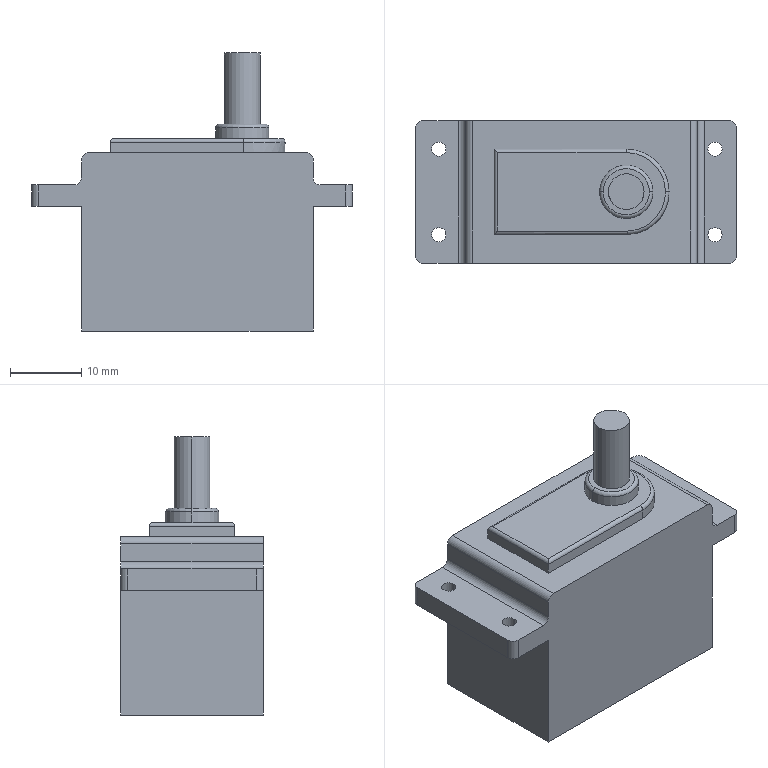Part | SolidWorks | features ICE 6, Fillet 2, Extrusion 1, Scale 1 | 1 solid | 48 faces | box 45 x 20 x 39 mm | volume 17798 mm3 | cylinder 24 | plane 20 | torus 4 | commonest cylinder face diameters 2 x16 1 x3 5 x2 7.5 x2 12 x1
STEP:
#1=CARTESIAN_POINT('',(17.75,6.,17.5));
#2=VERTEX_POINT('',#1);
#3=CARTESIAN_POINT('',(19.75,6.,17.5));
#4=VERTEX_POINT('',#3);
#5=CARTESIAN_POINT('',(18.75,6.,17.5));
#6=DIRECTION('',(0.,0.,1.));
#7=DIRECTION('',(0.,-1.,0.));
#8=AXIS2_PLACEMENT_3D('',#5,#6,#7);
#9=CIRCLE('',#8,1.);
#10=EDGE_CURVE('',#2,#4,#9,.T.);
#11=ORIENTED_EDGE('',*,*,#10,.F.);
#12=CARTESIAN_POINT('',(17.75,6.,20.5));
#13=VERTEX_POINT('',#12);
#14=CARTESIAN_POINT('',(17.75,6.,10.5));
#15=DIRECTION('',(0.,0.,1.));
#16=VECTOR('',#15,1000.);
#17=LINE('',#14,#16);
#18=EDGE_CURVE('',#2,#13,#17,.T.);
#19=ORIENTED_EDGE('',*,*,#18,.T.);
#20=CARTESIAN_POINT('',(19.75,6.,20.5));
#21=VERTEX_POINT('',#20);
#22=CARTESIAN_POINT('',(18.75,6.,20.5));
#23=DIRECTION('',(0.,0.,1.));
#24=DIRECTION('',(1.,0.,0.));
#25=AXIS2_PLACEMENT_3D('',#22,#23,#24);
#26=CIRCLE('',#25,1.);
#27=EDGE_CURVE('',#13,#21,#26,.T.);
#28=ORIENTED_EDGE('',*,*,#27,.T.);
#29=CARTESIAN_POINT('',(19.75,6.,10.5));
#30=DIRECTION('',(0.,0.,1.));
#31=VECTOR('',#30,1000.);
#32=LINE('',#29,#31);
#33=EDGE_CURVE('',#4,#21,#32,.T.);
#34=ORIENTED_EDGE('',*,*,#33,.F.);
#35=EDGE_LOOP('',(#11,#19,#28,#34));
#36=FACE_OUTER_BOUND('',#35,.T.);
#37=CARTESIAN_POINT('',(18.75,6.,10.5));
#38=DIRECTION('',(0.,0.,1.));
#39=DIRECTION('',(1.,0.,0.));
#40=AXIS2_PLACEMENT_3D('',#37,#38,#39);
#41=CYLINDRICAL_SURFACE('',#40,1.);
#42=ADVANCED_FACE('',(#36),#41,.F.);
#43=CARTESIAN_POINT('',(17.75,-6.,17.5));
#44=VERTEX_POINT('',#43);
#45=CARTESIAN_POINT('',(19.75,-6.,17.5));
#46=VERTEX_POINT('',#45);
#47=CARTESIAN_POINT('',(18.75,-6.,17.5));
#48=DIRECTION('',(0.,0.,1.));
#49=DIRECTION('',(0.,-1.,0.));
#50=AXIS2_PLACEMENT_3D('',#47,#48,#49);
#51=CIRCLE('',#50,1.);
#52=EDGE_CURVE('',#44,#46,#51,.T.);
#53=ORIENTED_EDGE('',*,*,#52,.F.);
#54=CARTESIAN_POINT('',(17.75,-6.,20.5));
#55=VERTEX_POINT('',#54);
#56=CARTESIAN_POINT('',(17.75,-6.,10.5));
#57=DIRECTION('',(0.,0.,1.));
#58=VECTOR('',#57,1000.);
#59=LINE('',#56,#58);
#60=EDGE_CURVE('',#44,#55,#59,.T.);
#61=ORIENTED_EDGE('',*,*,#60,.T.);
#62=CARTESIAN_POINT('',(19.75,-6.,20.5));
#63=VERTEX_POINT('',#62);
#64=CARTESIAN_POINT('',(18.75,-6.,20.5));
#65=DIRECTION('',(0.,0.,1.));
#66=DIRECTION('',(1.,0.,0.));
#67=AXIS2_PLACEMENT_3D('',#64,#65,#66);
#68=CIRCLE('',#67,1.);
#69=EDGE_CURVE('',#55,#63,#68,.T.);
#70=ORIENTED_EDGE('',*,*,#69,.T.);
#71=CARTESIAN_POINT('',(19.75,-6.,10.5));
#72=DIRECTION('',(0.,0.,1.));
#73=VECTOR('',#72,1000.);
#74=LINE('',#71,#73);
#75=EDGE_CURVE('',#46,#63,#74,.T.);
#76=ORIENTED_EDGE('',*,*,#75,.F.);
#77=EDGE_LOOP('',(#53,#61,#70,#76));
#78=FACE_OUTER_BOUND('',#77,.T.);
#79=CARTESIAN_POINT('',(18.75,-6.,10.5));
#80=DIRECTION('',(0.,0.,1.));
#81=DIRECTION('',(1.,0.,0.));
#82=AXIS2_PLACEMENT_3D('',#79,#80,#81);
#83=CYLINDRICAL_SURFACE('',#82,1.);
#84=ADVANCED_FACE('',(#78),#83,.F.);
#85=CARTESIAN_POINT('',(-20.99,-6.,17.5));
#86=VERTEX_POINT('',#85);
#87=CARTESIAN_POINT('',(-18.99,-6.,17.5));
#88=VERTEX_POINT('',#87);
#89=CARTESIAN_POINT('',(-19.99,-6.,17.5));
#90=DIRECTION('',(0.,0.,1.));
#91=DIRECTION('',(0.,-1.,0.));
#92=AXIS2_PLACEMENT_3D('',#89,#90,#91);
#93=CIRCLE('',#92,1.);
#94=EDGE_CURVE('',#86,#88,#93,.T.);
#95=ORIENTED_EDGE('',*,*,#94,.F.);
#96=CARTESIAN_POINT('',(-20.99,-6.,20.5));
#97=VERTEX_POINT('',#96);
#98=CARTESIAN_POINT('',(-20.99,-6.,10.5));
#99=DIRECTION('',(0.,0.,1.));
#100=VECTOR('',#99,1000.);
#101=LINE('',#98,#100);
#102=EDGE_CURVE('',#86,#97,#101,.T.);
#103=ORIENTED_EDGE('',*,*,#102,.T.);
#104=CARTESIAN_POINT('',(-18.99,-6.,20.5));
#105=VERTEX_POINT('',#104);
#106=CARTESIAN_POINT('',(-19.99,-6.,20.5));
#107=DIRECTION('',(0.,0.,1.));
#108=DIRECTION('',(1.,0.,0.));
#109=AXIS2_PLACEMENT_3D('',#106,#107,#108);
#110=CIRCLE('',#109,1.);
#111=EDGE_CURVE('',#97,#105,#110,.T.);
#112=ORIENTED_EDGE('',*,*,#111,.T.);
#113=CARTESIAN_POINT('',(-18.99,-6.,10.5));
#114=DIRECTION('',(0.,0.,1.));
#115=VECTOR('',#114,1000.);
#116=LINE('',#113,#115);
#117=EDGE_CURVE('',#88,#105,#116,.T.);
#118=ORIENTED_EDGE('',*,*,#117,.F.);
#119=EDGE_LOOP('',(#95,#103,#112,#118));
#120=FACE_OUTER_BOUND('',#119,.T.);
#121=CARTESIAN_POINT('',(-19.99,-6.,10.5));
#122=DIRECTION('',(0.,0.,1.));
#123=DIRECTION('',(1.,0.,0.));
#124=AXIS2_PLACEMENT_3D('',#121,#122,#123);
#125=CYLINDRICAL_SURFACE('',#124,1.);
#126=ADVANCED_FACE('',(#120),#125,.F.);
#127=CARTESIAN_POINT('',(-20.99,6.,17.5));
#128=VERTEX_POINT('',#127);
#129=CARTESIAN_POINT('',(-18.99,6.,17.5));
#130=VERTEX_POINT('',#129);
#131=CARTESIAN_POINT('',(-19.99,6.,17.5));
#132=DIRECTION('',(0.,0.,1.));
#133=DIRECTION('',(0.,-1.,0.));
#134=AXIS2_PLACEMENT_3D('',#131,#132,#133);
#135=CIRCLE('',#134,1.);
#136=EDGE_CURVE('',#128,#130,#135,.T.);
#137=ORIENTED_EDGE('',*,*,#136,.F.);
#138=CARTESIAN_POINT('',(-20.99,6.,20.5));
#139=VERTEX_POINT('',#138);
#140=CARTESIAN_POINT('',(-20.99,6.,10.5));
#141=DIRECTION('',(0.,0.,1.));
#142=VECTOR('',#141,1000.);
#143=LINE('',#140,#142);
#144=EDGE_CURVE('',#128,#139,#143,.T.);
#145=ORIENTED_EDGE('',*,*,#144,.T.);
#146=CARTESIAN_POINT('',(-18.99,6.,20.5));
#147=VERTEX_POINT('',#146);
#148=CARTESIAN_POINT('',(-19.99,6.,20.5));
#149=DIRECTION('',(0.,0.,1.));
#150=DIRECTION('',(1.,0.,0.));
#151=AXIS2_PLACEMENT_3D('',#148,#149,#150);
#152=CIRCLE('',#151,1.);
#153=EDGE_CURVE('',#139,#147,#152,.T.);
#154=ORIENTED_EDGE('',*,*,#153,.T.);
#155=CARTESIAN_POINT('',(-18.99,6.,10.5));
#156=DIRECTION('',(0.,0.,1.));
#157=VECTOR('',#156,1000.);
#158=LINE('',#155,#157);
#159=EDGE_CURVE('',#130,#147,#158,.T.);
#160=ORIENTED_EDGE('',*,*,#159,.F.);
#161=EDGE_LOOP('',(#137,#145,#154,#160));
#162=FACE_OUTER_BOUND('',#161,.T.);
#163=CARTESIAN_POINT('',(-19.99,6.,10.5));
#164=DIRECTION('',(0.,0.,1.));
#165=DIRECTION('',(1.,0.,0.));
#166=AXIS2_PLACEMENT_3D('',#163,#164,#165);
#167=CYLINDRICAL_SURFACE('',#166,1.);
#168=ADVANCED_FACE('',(#162),#167,.F.);
#169=CARTESIAN_POINT('',(2.551,0.,28.5));
#170=VERTEX_POINT('',#169);
#171=CARTESIAN_POINT('',(10.051,0.,28.5));
#172=VERTEX_POINT('',#171);
#173=CARTESIAN_POINT('',(6.301,0.,28.5));
#174=DIRECTION('',(0.,0.,-1.));
#175=DIRECTION('',(1.,0.,0.));
#176=AXIS2_PLACEMENT_3D('',#173,#174,#175);
#177=CIRCLE('',#176,3.75);
#178=EDGE_CURVE('',#170,#172,#177,.T.);
#179=ORIENTED_EDGE('',*,*,#178,.F.);
#180=CARTESIAN_POINT('',(3.051,0.,29.));
#181=VERTEX_POINT('',#180);
#182=CARTESIAN_POINT('',(3.051,0.,28.5));
#183=DIRECTION('',(0.,1.,0.));
#184=DIRECTION('',(-1.,0.,0.));
#185=AXIS2_PLACEMENT_3D('',#182,#183,#184);
#186=CIRCLE('',#185,0.5);
#187=EDGE_CURVE('',#170,#181,#186,.T.);
#188=ORIENTED_EDGE('',*,*,#187,.T.);
#189=CARTESIAN_POINT('',(9.551,0.,29.));
#190=VERTEX_POINT('',#189);
#191=CARTESIAN_POINT('',(6.301,0.,29.));
#192=DIRECTION('',(0.,0.,1.));
#193=DIRECTION('',(1.,0.,0.));
#194=AXIS2_PLACEMENT_3D('',#191,#192,#193);
#195=CIRCLE('',#194,3.25);
#196=EDGE_CURVE('',#190,#181,#195,.T.);
#197=ORIENTED_EDGE('',*,*,#196,.F.);
#198=CARTESIAN_POINT('',(9.551,0.,28.5));
#199=DIRECTION('',(0.,-1.,0.));
#200=DIRECTION('',(0.,0.,-1.));
#201=AXIS2_PLACEMENT_3D('',#198,#199,#200);
#202=CIRCLE('',#201,0.5);
#203=EDGE_CURVE('',#172,#190,#202,.T.);
#204=ORIENTED_EDGE('',*,*,#203,.F.);
#205=EDGE_LOOP('',(#179,#188,#197,#204));
#206=FACE_OUTER_BOUND('',#205,.T.);
#207=CARTESIAN_POINT('',(6.301,0.,28.5));
#208=DIRECTION('',(0.,0.,1.));
#209=DIRECTION('',(1.,0.,0.));
#210=AXIS2_PLACEMENT_3D('',#207,#208,#209);
#211=TOROIDAL_SURFACE('',#210,3.25,0.5);
#212=ADVANCED_FACE('',(#206),#211,.T.);
#213=CARTESIAN_POINT('',(12.301,0.,26.5));
#214=VERTEX_POINT('',#213);
#215=CARTESIAN_POINT('',(6.498,-5.997,26.5));
#216=VERTEX_POINT('',#215);
#217=CARTESIAN_POINT('',(6.301,0.,26.5));
#218=DIRECTION('',(0.,0.,-1.));
#219=DIRECTION('',(1.,0.,0.));
#220=AXIS2_PLACEMENT_3D('',#217,#218,#219);
#221=CIRCLE('',#220,6.);
#222=EDGE_CURVE('',#214,#216,#221,.T.);
#223=ORIENTED_EDGE('',*,*,#222,.F.);
#224=CARTESIAN_POINT('',(11.801,0.,27.));
#225=VERTEX_POINT('',#224);
#226=CARTESIAN_POINT('',(11.801,0.,26.5));
#227=DIRECTION('',(0.,-1.,0.));
#228=DIRECTION('',(0.,0.,-1.));
#229=AXIS2_PLACEMENT_3D('',#226,#227,#228);
#230=CIRCLE('',#229,0.5);
#231=EDGE_CURVE('',#214,#225,#230,.T.);
#232=ORIENTED_EDGE('',*,*,#231,.T.);
#233=CARTESIAN_POINT('',(6.489,-5.497,27.));
#234=VERTEX_POINT('',#233);
#235=CARTESIAN_POINT('',(6.301,0.,27.));
#236=DIRECTION('',(0.,0.,1.));
#237=DIRECTION('',(1.,0.,0.));
#238=AXIS2_PLACEMENT_3D('',#235,#236,#237);
#239=CIRCLE('',#238,5.5);
#240=EDGE_CURVE('',#234,#225,#239,.T.);
#241=ORIENTED_EDGE('',*,*,#240,.F.);
#242=CARTESIAN_POINT('',(6.489,-5.497,27.));
#243=CARTESIAN_POINT('',(6.492,-5.628,27.));
#244=CARTESIAN_POINT('',(6.494,-5.758,26.946));
#245=CARTESIAN_POINT('',(6.497,-5.943,26.761));
#246=CARTESIAN_POINT('',(6.498,-5.997,26.632));
#247=CARTESIAN_POINT('',(6.498,-5.997,26.5));
#248=B_SPLINE_CURVE_WITH_KNOTS('',3,(#242,#243,#244,#245,#246,#247),.UNSPECIFIED.,.F.,.F.,(4,2,4),(-0.00001713,0.0003773,0.0007717),.UNSPECIFIED.);
#249=EDGE_CURVE('',#234,#216,#248,.T.);
#250=ORIENTED_EDGE('',*,*,#249,.T.);
#251=EDGE_LOOP('',(#223,#232,#241,#250));
#252=FACE_OUTER_BOUND('',#251,.T.);
#253=CARTESIAN_POINT('',(6.301,0.,26.5));
#254=DIRECTION('',(0.,0.,1.));
#255=DIRECTION('',(1.,0.,0.));
#256=AXIS2_PLACEMENT_3D('',#253,#254,#255);
#257=TOROIDAL_SURFACE('',#256,5.5,0.5);
#258=ADVANCED_FACE('',(#252),#257,.T.);
#259=CARTESIAN_POINT('',(8.801,0.,39.));
#260=VERTEX_POINT('',#259);
#261=CARTESIAN_POINT('',(3.801,0.,39.));
#262=VERTEX_POINT('',#261);
#263=CARTESIAN_POINT('',(6.301,0.,39.));
#264=DIRECTION('',(0.,0.,1.));
#265=DIRECTION('',(1.,0.,0.));
#266=AXIS2_PLACEMENT_3D('',#263,#264,#265);
#267=CIRCLE('',#266,2.5);
#268=EDGE_CURVE('',#260,#262,#267,.T.);
#269=ORIENTED_EDGE('',*,*,#268,.F.);
#270=CARTESIAN_POINT('',(8.801,0.,29.));
#271=VERTEX_POINT('',#270);
#272=CARTESIAN_POINT('',(8.801,0.,39.));
#273=DIRECTION('',(0.,0.,-1.));
#274=VECTOR('',#273,1000.);
#275=LINE('',#272,#274);
#276=EDGE_CURVE('',#260,#271,#275,.T.);
#277=ORIENTED_EDGE('',*,*,#276,.T.);
#278=CARTESIAN_POINT('',(3.801,0.,29.));
#279=VERTEX_POINT('',#278);
#280=CARTESIAN_POINT('',(6.301,0.,29.));
#281=DIRECTION('',(0.,0.,1.));
#282=DIRECTION('',(1.,0.,0.));
#283=AXIS2_PLACEMENT_3D('',#280,#281,#282);
#284=CIRCLE('',#283,2.5);
#285=EDGE_CURVE('',#271,#279,#284,.T.);
#286=ORIENTED_EDGE('',*,*,#285,.T.);
#287=CARTESIAN_POINT('',(3.801,0.,39.));
#288=DIRECTION('',(0.,0.,-1.));
#289=VECTOR('',#288,1000.);
#290=LINE('',#287,#289);
#291=EDGE_CURVE('',#262,#279,#290,.T.);
#292=ORIENTED_EDGE('',*,*,#291,.F.);
#293=EDGE_LOOP('',(#269,#277,#286,#292));
#294=FACE_OUTER_BOUND('',#293,.T.);
#295=CARTESIAN_POINT('',(6.301,0.,39.));
#296=DIRECTION('',(0.,0.,-1.));
#297=DIRECTION('',(-1.,0.,0.));
#298=AXIS2_PLACEMENT_3D('',#295,#296,#297);
#299=CYLINDRICAL_SURFACE('',#298,2.5);
#300=ADVANCED_FACE('',(#294),#299,.T.);
#301=ORIENTED_EDGE('',*,*,#178,.T.);
#302=CARTESIAN_POINT('',(10.051,0.,27.));
#303=VERTEX_POINT('',#302);
#304=CARTESIAN_POINT('',(10.051,0.,29.));
#305=DIRECTION('',(0.,0.,-1.));
#306=VECTOR('',#305,1000.);
#307=LINE('',#304,#306);
#308=EDGE_CURVE('',#172,#303,#307,.T.);
#309=ORIENTED_EDGE('',*,*,#308,.T.);
#310=CARTESIAN_POINT('',(2.551,0.,27.));
#311=VERTEX_POINT('',#310);
#312=CARTESIAN_POINT('',(6.301,0.,27.));
#313=DIRECTION('',(0.,0.,1.));
#314=DIRECTION('',(1.,0.,0.));
#315=AXIS2_PLACEMENT_3D('',#312,#313,#314);
#316=CIRCLE('',#315,3.75);
#317=EDGE_CURVE('',#303,#311,#316,.T.);
#318=ORIENTED_EDGE('',*,*,#317,.T.);
#319=CARTESIAN_POINT('',(2.551,0.,29.));
#320=DIRECTION('',(0.,0.,-1.));
#321=VECTOR('',#320,1000.);
#322=LINE('',#319,#321);
#323=EDGE_CURVE('',#170,#311,#322,.T.);
#324=ORIENTED_EDGE('',*,*,#323,.F.);
#325=EDGE_LOOP('',(#301,#309,#318,#324));
#326=FACE_OUTER_BOUND('',#325,.T.);
#327=CARTESIAN_POINT('',(6.301,0.,29.));
#328=DIRECTION('',(0.,0.,-1.));
#329=DIRECTION('',(-1.,0.,0.));
#330=AXIS2_PLACEMENT_3D('',#327,#328,#329);
#331=CYLINDRICAL_SURFACE('',#330,3.75);
#332=ADVANCED_FACE('',(#326),#331,.T.);
#333=CARTESIAN_POINT('',(-16.25,10.,24.));
#334=VERTEX_POINT('',#333);
#335=CARTESIAN_POINT('',(-16.25,10.,21.5));
#336=VERTEX_POINT('',#335);
#337=CARTESIAN_POINT('',(-16.25,10.,25.));
#338=DIRECTION('',(0.,0.,-1.));
#339=VECTOR('',#338,1000.);
#340=LINE('',#337,#339);
#341=EDGE_CURVE('',#334,#336,#340,.T.);
#342=ORIENTED_EDGE('',*,*,#341,.T.);
#343=CARTESIAN_POINT('',(-16.25,-10.,21.5));
#344=VERTEX_POINT('',#343);
#345=CARTESIAN_POINT('',(-16.25,-10.,21.5));
#346=DIRECTION('',(0.,-1.,0.));
#347=VECTOR('',#346,1000.);
#348=LINE('',#345,#347);
#349=EDGE_CURVE('',#336,#344,#348,.T.);
#350=ORIENTED_EDGE('',*,*,#349,.T.);
#351=CARTESIAN_POINT('',(-16.25,-10.,24.));
#352=VERTEX_POINT('',#351);
#353=CARTESIAN_POINT('',(-16.25,-10.,25.));
#354=DIRECTION('',(0.,0.,-1.));
#355=VECTOR('',#354,1000.);
#356=LINE('',#353,#355);
#357=EDGE_CURVE('',#352,#344,#356,.T.);
#358=ORIENTED_EDGE('',*,*,#357,.F.);
#359=CARTESIAN_POINT('',(-16.25,10.,24.));
#360=DIRECTION('',(0.,1.,0.));
#361=VECTOR('',#360,1000.);
#362=LINE('',#359,#361);
#363=EDGE_CURVE('',#352,#334,#362,.T.);
#364=ORIENTED_EDGE('',*,*,#363,.T.);
#365=EDGE_LOOP('',(#342,#350,#358,#364));
#366=FACE_OUTER_BOUND('',#365,.T.);
#367=CARTESIAN_POINT('',(-16.25,-10.,25.));
#368=DIRECTION('',(1.,0.,0.));
#369=DIRECTION('',(0.,0.,-1.));
#370=AXIS2_PLACEMENT_3D('',#367,#368,#369);
#371=PLANE('',#370);
#372=ADVANCED_FACE('',(#366),#371,.F.);
#373=CARTESIAN_POINT('',(-16.25,10.,17.5));
#374=VERTEX_POINT('',#373);
#375=CARTESIAN_POINT('',(-16.25,-10.,17.5));
#376=VERTEX_POINT('',#375);
#377=CARTESIAN_POINT('',(-16.25,10.,17.5));
#378=DIRECTION('',(0.,-1.,0.));
#379=VECTOR('',#378,1000.);
#380=LINE('',#377,#379);
#381=EDGE_CURVE('',#374,#376,#380,.T.);
#382=ORIENTED_EDGE('',*,*,#381,.F.);
#383=CARTESIAN_POINT('',(-16.25,10.,0.));
#384=VERTEX_POINT('',#383);
#385=CARTESIAN_POINT('',(-16.25,10.,25.));
#386=DIRECTION('',(0.,0.,-1.));
#387=VECTOR('',#386,1000.);
#388=LINE('',#385,#387);
#389=EDGE_CURVE('',#374,#384,#388,.T.);
#390=ORIENTED_EDGE('',*,*,#389,.T.);
#391=CARTESIAN_POINT('',(-16.25,-10.,0.));
#392=VERTEX_POINT('',#391);
#393=CARTESIAN_POINT('',(-16.25,-10.,0.));
#394=DIRECTION('',(0.,-1.,0.));
#395=VECTOR('',#394,1000.);
#396=LINE('',#393,#395);
#397=EDGE_CURVE('',#384,#392,#396,.T.);
#398=ORIENTED_EDGE('',*,*,#397,.T.);
#399=CARTESIAN_POINT('',(-16.25,-10.,25.));
#400=DIRECTION('',(0.,0.,-1.));
#401=VECTOR('',#400,1000.);
#402=LINE('',#399,#401);
#403=EDGE_CURVE('',#376,#392,#402,.T.);
#404=ORIENTED_EDGE('',*,*,#403,.F.);
#405=EDGE_LOOP('',(#382,#390,#398,#404));
#406=FACE_OUTER_BOUND('',#405,.T.);
#407=CARTESIAN_POINT('',(-16.25,-10.,25.));
#408=DIRECTION('',(1.,0.,0.));
#409=DIRECTION('',(0.,0.,-1.));
#410=AXIS2_PLACEMENT_3D('',#407,#408,#409);
#411=PLANE('',#410);
#412=ADVANCED_FACE('',(#406),#411,.F.);
#413=CARTESIAN_POINT('',(16.25,-10.,24.));
#414=VERTEX_POINT('',#413);
#415=CARTESIAN_POINT('',(16.25,-10.,21.5));
#416=VERTEX_POINT('',#415);
#417=CARTESIAN_POINT('',(16.25,-10.,25.));
#418=DIRECTION('',(0.,0.,-1.));
#419=VECTOR('',#418,1000.);
#420=LINE('',#417,#419);
#421=EDGE_CURVE('',#414,#416,#420,.T.);
#422=ORIENTED_EDGE('',*,*,#421,.T.);
#423=CARTESIAN_POINT('',(16.25,10.,21.5));
#424=VERTEX_POINT('',#423);
#425=CARTESIAN_POINT('',(16.25,10.,21.5));
#426=DIRECTION('',(0.,1.,0.));
#427=VECTOR('',#426,1000.);
#428=LINE('',#425,#427);
#429=EDGE_CURVE('',#416,#424,#428,.T.);
#430=ORIENTED_EDGE('',*,*,#429,.T.);
#431=CARTESIAN_POINT('',(16.25,10.,24.));
#432=VERTEX_POINT('',#431);
#433=CARTESIAN_POINT('',(16.25,10.,25.));
#434=DIRECTION('',(0.,0.,-1.));
#435=VECTOR('',#434,1000.);
#436=LINE('',#433,#435);
#437=EDGE_CURVE('',#432,#424,#436,.T.);
#438=ORIENTED_EDGE('',*,*,#437,.F.);
#439=CARTESIAN_POINT('',(16.25,-10.,24.));
#440=DIRECTION('',(0.,-1.,0.));
#441=VECTOR('',#440,1000.);
#442=LINE('',#439,#441);
#443=EDGE_CURVE('',#432,#414,#442,.T.);
#444=ORIENTED_EDGE('',*,*,#443,.T.);
#445=EDGE_LOOP('',(#422,#430,#438,#444));
#446=FACE_OUTER_BOUND('',#445,.T.);
#447=CARTESIAN_POINT('',(16.25,-10.,25.));
#448=DIRECTION('',(-1.,0.,0.));
#449=DIRECTION('',(0.,0.,1.));
#450=AXIS2_PLACEMENT_3D('',#447,#448,#449);
#451=PLANE('',#450);
#452=ADVANCED_FACE('',(#446),#451,.F.);
#453=CARTESIAN_POINT('',(16.25,-10.,17.5));
#454=VERTEX_POINT('',#453);
#455=CARTESIAN_POINT('',(16.25,10.,17.5));
#456=VERTEX_POINT('',#455);
#457=CARTESIAN_POINT('',(16.25,10.,17.5));
#458=DIRECTION('',(0.,1.,0.));
#459=VECTOR('',#458,1000.);
#460=LINE('',#457,#459);
#461=EDGE_CURVE('',#454,#456,#460,.T.);
#462=ORIENTED_EDGE('',*,*,#461,.F.);
#463=CARTESIAN_POINT('',(16.25,-10.,0.));
#464=VERTEX_POINT('',#463);
#465=CARTESIAN_POINT('',(16.25,-10.,25.));
#466=DIRECTION('',(0.,0.,-1.));
#467=VECTOR('',#466,1000.);
#468=LINE('',#465,#467);
#469=EDGE_CURVE('',#454,#464,#468,.T.);
#470=ORIENTED_EDGE('',*,*,#469,.T.);
#471=CARTESIAN_POINT('',(16.25,10.,0.));
#472=VERTEX_POINT('',#471);
#473=CARTESIAN_POINT('',(16.25,-10.,0.));
#474=DIRECTION('',(0.,1.,0.));
#475=VECTOR('',#474,1000.);
#476=LINE('',#473,#475);
#477=EDGE_CURVE('',#464,#472,#476,.T.);
#478=ORIENTED_EDGE('',*,*,#477,.T.);
#479=CARTESIAN_POINT('',(16.25,10.,25.));
#480=DIRECTION('',(0.,0.,-1.));
#481=VECTOR('',#480,1000.);
#482=LINE('',#479,#481);
#483=EDGE_CURVE('',#456,#472,#482,.T.);
#484=ORIENTED_EDGE('',*,*,#483,.F.);
#485=EDGE_LOOP('',(#462,#470,#478,#484));
#486=FACE_OUTER_BOUND('',#485,.T.);
#487=CARTESIAN_POINT('',(16.25,-10.,25.));
#488=DIRECTION('',(-1.,0.,0.));
#489=DIRECTION('',(0.,0.,1.));
#490=AXIS2_PLACEMENT_3D('',#487,#488,#489);
#491=PLANE('',#490);
#492=ADVANCED_FACE('',(#486),#491,.F.);
#493=ORIENTED_EDGE('',*,*,#421,.F.);
#494=CARTESIAN_POINT('',(15.25,-10.,25.));
#495=VERTEX_POINT('',#494);
#496=CARTESIAN_POINT('',(15.25,-10.,24.));
#497=DIRECTION('',(0.,-1.,0.));
#498=DIRECTION('',(-1.,0.,0.));
#499=AXIS2_PLACEMENT_3D('',#496,#497,#498);
#500=CIRCLE('',#499,1.);
#501=EDGE_CURVE('',#414,#495,#500,.T.);
#502=ORIENTED_EDGE('',*,*,#501,.T.);
#503=CARTESIAN_POINT('',(-15.25,-10.,25.));
#504=VERTEX_POINT('',#503);
#505=CARTESIAN_POINT('',(16.25,-10.,25.));
#506=DIRECTION('',(1.,0.,0.));
#507=VECTOR('',#506,1000.);
#508=LINE('',#505,#507);
#509=EDGE_CURVE('',#504,#495,#508,.T.);
#510=ORIENTED_EDGE('',*,*,#509,.F.);
#511=CARTESIAN_POINT('',(-15.25,-10.,24.));
#512=DIRECTION('',(0.,-1.,0.));
#513=DIRECTION('',(-1.,0.,0.));
#514=AXIS2_PLACEMENT_3D('',#511,#512,#513);
#515=CIRCLE('',#514,1.);
#516=EDGE_CURVE('',#504,#352,#515,.T.);
#517=ORIENTED_EDGE('',*,*,#516,.T.);
#518=ORIENTED_EDGE('',*,*,#357,.T.);
#519=CARTESIAN_POINT('',(-17.25,-10.,20.5));
#520=VERTEX_POINT('',#519);
#521=CARTESIAN_POINT('',(-17.25,-10.,21.5));
#522=DIRECTION('',(0.,1.,0.));
#523=DIRECTION('',(-1.,0.,0.));
#524=AXIS2_PLACEMENT_3D('',#521,#522,#523);
#525=CIRCLE('',#524,1.);
#526=EDGE_CURVE('',#344,#520,#525,.T.);
#527=ORIENTED_EDGE('',*,*,#526,.T.);
#528=CARTESIAN_POINT('',(-22.25,-10.,20.5));
#529=VERTEX_POINT('',#528);
#530=CARTESIAN_POINT('',(-26.25,-10.,20.5));
#531=DIRECTION('',(1.,0.,0.));
#532=VECTOR('',#531,1000.);
#533=LINE('',#530,#532);
#534=EDGE_CURVE('',#529,#520,#533,.T.);
#535=ORIENTED_EDGE('',*,*,#534,.F.);
#536=CARTESIAN_POINT('',(-22.25,-10.,17.5));
#537=VERTEX_POINT('',#536);
#538=CARTESIAN_POINT('',(-22.25,-10.,25.));
#539=DIRECTION('',(0.,0.,-1.));
#540=VECTOR('',#539,1000.);
#541=LINE('',#538,#540);
#542=EDGE_CURVE('',#529,#537,#541,.T.);
#543=ORIENTED_EDGE('',*,*,#542,.T.);
#544=CARTESIAN_POINT('',(-26.25,-10.,17.5));
#545=DIRECTION('',(1.,0.,0.));
#546=VECTOR('',#545,1000.);
#547=LINE('',#544,#546);
#548=EDGE_CURVE('',#537,#376,#547,.T.);
#549=ORIENTED_EDGE('',*,*,#548,.T.);
#550=ORIENTED_EDGE('',*,*,#403,.T.);
#551=CARTESIAN_POINT('',(16.25,-10.,0.));
#552=DIRECTION('',(1.,0.,0.));
#553=VECTOR('',#552,1000.);
#554=LINE('',#551,#553);
#555=EDGE_CURVE('',#392,#464,#554,.T.);
#556=ORIENTED_EDGE('',*,*,#555,.T.);
#557=ORIENTED_EDGE('',*,*,#469,.F.);
#558=CARTESIAN_POINT('',(20.75,-10.,17.5));
#559=VERTEX_POINT('',#558);
#560=CARTESIAN_POINT('',(26.25,-10.,17.5));
#561=DIRECTION('',(-1.,0.,0.));
#562=VECTOR('',#561,1000.);
#563=LINE('',#560,#562);
#564=EDGE_CURVE('',#559,#454,#563,.T.);
#565=ORIENTED_EDGE('',*,*,#564,.F.);
#566=CARTESIAN_POINT('',(20.75,-10.,20.5));
#567=VERTEX_POINT('',#566);
#568=CARTESIAN_POINT('',(20.75,-10.,25.));
#569=DIRECTION('',(0.,0.,1.));
#570=VECTOR('',#569,1000.);
#571=LINE('',#568,#570);
#572=EDGE_CURVE('',#559,#567,#571,.T.);
#573=ORIENTED_EDGE('',*,*,#572,.T.);
#574=CARTESIAN_POINT('',(17.25,-10.,20.5));
#575=VERTEX_POINT('',#574);
#576=CARTESIAN_POINT('',(26.25,-10.,20.5));
#577=DIRECTION('',(-1.,0.,0.));
#578=VECTOR('',#577,1000.);
#579=LINE('',#576,#578);
#580=EDGE_CURVE('',#567,#575,#579,.T.);
#581=ORIENTED_EDGE('',*,*,#580,.T.);
#582=CARTESIAN_POINT('',(17.25,-10.,21.5));
#583=DIRECTION('',(0.,1.,0.));
#584=DIRECTION('',(-1.,0.,0.));
#585=AXIS2_PLACEMENT_3D('',#582,#583,#584);
#586=CIRCLE('',#585,1.);
#587=EDGE_CURVE('',#575,#416,#586,.T.);
#588=ORIENTED_EDGE('',*,*,#587,.T.);
#589=EDGE_LOOP('',(#493,#502,#510,#517,#518,#527,#535,#543,#549,#550,#556,#557,#565,#573,#581,#588));
#590=FACE_OUTER_BOUND('',#589,.T.);
#591=CARTESIAN_POINT('',(16.25,-10.,25.));
#592=DIRECTION('',(0.,1.,0.));
#593=DIRECTION('',(-1.,0.,0.));
#594=AXIS2_PLACEMENT_3D('',#591,#592,#593);
#595=PLANE('',#594);
#596=ADVANCED_FACE('',(#590),#595,.F.);
#597=CARTESIAN_POINT('',(15.25,10.,25.));
#598=VERTEX_POINT('',#597);
#599=CARTESIAN_POINT('',(-15.25,10.,25.));
#600=VERTEX_POINT('',#599);
#601=CARTESIAN_POINT('',(16.25,10.,25.));
#602=DIRECTION('',(-1.,0.,0.));
#603=VECTOR('',#602,1000.);
#604=LINE('',#601,#603);
#605=EDGE_CURVE('',#598,#600,#604,.T.);
#606=ORIENTED_EDGE('',*,*,#605,.F.);
#607=CARTESIAN_POINT('',(15.25,10.,24.));
#608=DIRECTION('',(0.,1.,0.));
#609=DIRECTION('',(1.,0.,0.));
#610=AXIS2_PLACEMENT_3D('',#607,#608,#609);
#611=CIRCLE('',#610,1.);
#612=EDGE_CURVE('',#598,#432,#611,.T.);
#613=ORIENTED_EDGE('',*,*,#612,.T.);
#614=ORIENTED_EDGE('',*,*,#437,.T.);
#615=CARTESIAN_POINT('',(17.25,10.,20.5));
#616=VERTEX_POINT('',#615);
#617=CARTESIAN_POINT('',(17.25,10.,21.5));
#618=DIRECTION('',(0.,-1.,0.));
#619=DIRECTION('',(1.,0.,0.));
#620=AXIS2_PLACEMENT_3D('',#617,#618,#619);
#621=CIRCLE('',#620,1.);
#622=EDGE_CURVE('',#424,#616,#621,.T.);
#623=ORIENTED_EDGE('',*,*,#622,.T.);
#624=CARTESIAN_POINT('',(20.75,10.,20.5));
#625=VERTEX_POINT('',#624);
#626=CARTESIAN_POINT('',(26.25,10.,20.5));
#627=DIRECTION('',(-1.,0.,0.));
#628=VECTOR('',#627,1000.);
#629=LINE('',#626,#628);
#630=EDGE_CURVE('',#625,#616,#629,.T.);
#631=ORIENTED_EDGE('',*,*,#630,.F.);
#632=CARTESIAN_POINT('',(20.75,10.,17.5));
#633=VERTEX_POINT('',#632);
#634=CARTESIAN_POINT('',(20.75,10.,25.));
#635=DIRECTION('',(0.,0.,-1.));
#636=VECTOR('',#635,1000.);
#637=LINE('',#634,#636);
#638=EDGE_CURVE('',#625,#633,#637,.T.);
#639=ORIENTED_EDGE('',*,*,#638,.T.);
#640=CARTESIAN_POINT('',(26.25,10.,17.5));
#641=DIRECTION('',(-1.,0.,0.));
#642=VECTOR('',#641,1000.);
#643=LINE('',#640,#642);
#644=EDGE_CURVE('',#633,#456,#643,.T.);
#645=ORIENTED_EDGE('',*,*,#644,.T.);
#646=ORIENTED_EDGE('',*,*,#483,.T.);
#647=CARTESIAN_POINT('',(16.25,10.,0.));
#648=DIRECTION('',(-1.,0.,0.));
#649=VECTOR('',#648,1000.);
#650=LINE('',#647,#649);
#651=EDGE_CURVE('',#472,#384,#650,.T.);
#652=ORIENTED_EDGE('',*,*,#651,.T.);
#653=ORIENTED_EDGE('',*,*,#389,.F.);
#654=CARTESIAN_POINT('',(-22.25,10.,17.5));
#655=VERTEX_POINT('',#654);
#656=CARTESIAN_POINT('',(-26.25,10.,17.5));
#657=DIRECTION('',(1.,0.,0.));
#658=VECTOR('',#657,1000.);
#659=LINE('',#656,#658);
#660=EDGE_CURVE('',#655,#374,#659,.T.);
#661=ORIENTED_EDGE('',*,*,#660,.F.);
#662=CARTESIAN_POINT('',(-22.25,10.,20.5));
#663=VERTEX_POINT('',#662);
#664=CARTESIAN_POINT('',(-22.25,10.,25.));
#665=DIRECTION('',(0.,0.,1.));
#666=VECTOR('',#665,1000.);
#667=LINE('',#664,#666);
#668=EDGE_CURVE('',#655,#663,#667,.T.);
#669=ORIENTED_EDGE('',*,*,#668,.T.);
#670=CARTESIAN_POINT('',(-17.25,10.,20.5));
#671=VERTEX_POINT('',#670);
#672=CARTESIAN_POINT('',(-26.25,10.,20.5));
#673=DIRECTION('',(1.,0.,0.));
#674=VECTOR('',#673,1000.);
#675=LINE('',#672,#674);
#676=EDGE_CURVE('',#663,#671,#675,.T.);
#677=ORIENTED_EDGE('',*,*,#676,.T.);
#678=CARTESIAN_POINT('',(-17.25,10.,21.5));
#679=DIRECTION('',(0.,-1.,0.));
#680=DIRECTION('',(1.,0.,0.));
#681=AXIS2_PLACEMENT_3D('',#678,#679,#680);
#682=CIRCLE('',#681,1.);
#683=EDGE_CURVE('',#671,#336,#682,.T.);
#684=ORIENTED_EDGE('',*,*,#683,.T.);
#685=ORIENTED_EDGE('',*,*,#341,.F.);
#686=CARTESIAN_POINT('',(-15.25,10.,24.));
#687=DIRECTION('',(0.,1.,0.));
#688=DIRECTION('',(1.,0.,0.));
#689=AXIS2_PLACEMENT_3D('',#686,#687,#688);
#690=CIRCLE('',#689,1.);
#691=EDGE_CURVE('',#334,#600,#690,.T.);
#692=ORIENTED_EDGE('',*,*,#691,.T.);
#693=EDGE_LOOP('',(#606,#613,#614,#623,#631,#639,#645,#646,#652,#653,#661,#669,#677,#684,#685,#692));
#694=FACE_OUTER_BOUND('',#693,.T.);
#695=CARTESIAN_POINT('',(16.25,10.,25.));
#696=DIRECTION('',(0.,-1.,0.));
#697=DIRECTION('',(1.,0.,0.));
#698=AXIS2_PLACEMENT_3D('',#695,#696,#697);
#699=PLANE('',#698);
#700=ADVANCED_FACE('',(#694),#699,.F.);
#701=CARTESIAN_POINT('',(-12.25,-6.,25.));
#702=VERTEX_POINT('',#701);
#703=CARTESIAN_POINT('',(6.498,-5.997,25.));
#704=VERTEX_POINT('',#703);
#705=CARTESIAN_POINT('',(0.00105,-5.998,25.));
#706=DIRECTION('',(1.,0.0001751,0.));
#707=VECTOR('',#706,1000.);
#708=LINE('',#705,#707);
#709=EDGE_CURVE('',#702,#704,#708,.T.);
#710=ORIENTED_EDGE('',*,*,#709,.F.);
#711=CARTESIAN_POINT('',(-12.25,6.,25.));
#712=VERTEX_POINT('',#711);
#713=CARTESIAN_POINT('',(-12.25,0.,25.));
#714=DIRECTION('',(0.,-1.,0.));
#715=VECTOR('',#714,1000.);
#716=LINE('',#713,#715);
#717=EDGE_CURVE('',#712,#702,#716,.T.);
#718=ORIENTED_EDGE('',*,*,#717,.F.);
#719=CARTESIAN_POINT('',(6.301,6.,25.));
#720=VERTEX_POINT('',#719);
#721=CARTESIAN_POINT('',(0.,6.,25.));
#722=DIRECTION('',(-1.,0.,0.));
#723=VECTOR('',#722,1000.);
#724=LINE('',#721,#723);
#725=EDGE_CURVE('',#720,#712,#724,.T.);
#726=ORIENTED_EDGE('',*,*,#725,.F.);
#727=CARTESIAN_POINT('',(6.301,0.,25.));
#728=DIRECTION('',(0.,0.,1.));
#729=DIRECTION('',(1.,0.,0.));
#730=AXIS2_PLACEMENT_3D('',#727,#728,#729);
#731=CIRCLE('',#730,6.);
#732=EDGE_CURVE('',#704,#720,#731,.T.);
#733=ORIENTED_EDGE('',*,*,#732,.F.);
#734=EDGE_LOOP('',(#710,#718,#726,#733));
#735=FACE_BOUND('',#734,.T.);
#736=ORIENTED_EDGE('',*,*,#509,.T.);
#737=CARTESIAN_POINT('',(15.25,10.,25.));
#738=DIRECTION('',(0.,1.,0.));
#739=VECTOR('',#738,1000.);
#740=LINE('',#737,#739);
#741=EDGE_CURVE('',#495,#598,#740,.T.);
#742=ORIENTED_EDGE('',*,*,#741,.T.);
#743=ORIENTED_EDGE('',*,*,#605,.T.);
#744=CARTESIAN_POINT('',(-15.25,-10.,25.));
#745=DIRECTION('',(0.,-1.,0.));
#746=VECTOR('',#745,1000.);
#747=LINE('',#744,#746);
#748=EDGE_CURVE('',#600,#504,#747,.T.);
#749=ORIENTED_EDGE('',*,*,#748,.T.);
#750=EDGE_LOOP('',(#736,#742,#743,#749));
#751=FACE_OUTER_BOUND('',#750,.T.);
#752=CARTESIAN_POINT('',(0.,0.,25.));
#753=DIRECTION('',(0.,0.,1.));
#754=DIRECTION('',(1.,0.,0.));
#755=AXIS2_PLACEMENT_3D('',#752,#753,#754);
#756=PLANE('',#755);
#757=ADVANCED_FACE('',(#735,#751),#756,.T.);
#758=ORIENTED_EDGE('',*,*,#397,.F.);
#759=ORIENTED_EDGE('',*,*,#651,.F.);
#760=ORIENTED_EDGE('',*,*,#477,.F.);
#761=ORIENTED_EDGE('',*,*,#555,.F.);
#762=EDGE_LOOP('',(#758,#759,#760,#761));
#763=FACE_OUTER_BOUND('',#762,.T.);
#764=CARTESIAN_POINT('',(0.,0.,0.));
#765=DIRECTION('',(0.,0.,1.));
#766=DIRECTION('',(1.,0.,0.));
#767=AXIS2_PLACEMENT_3D('',#764,#765,#766);
#768=PLANE('',#767);
#769=ADVANCED_FACE('',(#763),#768,.F.);
#770=CARTESIAN_POINT('',(6.498,-5.997,27.));
#771=DIRECTION('',(0.,0.,-1.));
#772=VECTOR('',#771,1000.);
#773=LINE('',#770,#772);
#774=EDGE_CURVE('',#216,#704,#773,.T.);
#775=ORIENTED_EDGE('',*,*,#774,.F.);
#776=CARTESIAN_POINT('',(-12.25,-6.,26.5));
#777=VERTEX_POINT('',#776);
#778=CARTESIAN_POINT('',(-12.25,-6.,26.5));
#779=DIRECTION('',(-1.,-0.0001751,0.));
#780=VECTOR('',#779,1000.);
#781=LINE('',#778,#780);
#782=EDGE_CURVE('',#216,#777,#781,.T.);
#783=ORIENTED_EDGE('',*,*,#782,.T.);
#784=CARTESIAN_POINT('',(-12.25,-6.,27.));
#785=DIRECTION('',(0.,0.,-1.));
#786=VECTOR('',#785,1000.);
#787=LINE('',#784,#786);
#788=EDGE_CURVE('',#777,#702,#787,.T.);
#789=ORIENTED_EDGE('',*,*,#788,.T.);
#790=ORIENTED_EDGE('',*,*,#709,.T.);
#791=EDGE_LOOP('',(#775,#783,#789,#790));
#792=FACE_OUTER_BOUND('',#791,.T.);
#793=CARTESIAN_POINT('',(0.00105,-5.998,27.));
#794=DIRECTION('',(-0.0001751,1.,0.));
#795=DIRECTION('',(-1.,-0.0001751,0.));
#796=AXIS2_PLACEMENT_3D('',#793,#794,#795);
#797=PLANE('',#796);
#798=ADVANCED_FACE('',(#792),#797,.F.);
#799=CARTESIAN_POINT('',(6.301,6.,26.5));
#800=VERTEX_POINT('',#799);
#801=CARTESIAN_POINT('',(6.301,6.,27.));
#802=DIRECTION('',(0.,0.,-1.));
#803=VECTOR('',#802,1000.);
#804=LINE('',#801,#803);
#805=EDGE_CURVE('',#800,#720,#804,.T.);
#806=ORIENTED_EDGE('',*,*,#805,.F.);
#807=CARTESIAN_POINT('',(6.301,0.,26.5));
#808=DIRECTION('',(0.,0.,-1.));
#809=DIRECTION('',(1.,0.,0.));
#810=AXIS2_PLACEMENT_3D('',#807,#808,#809);
#811=CIRCLE('',#810,6.);
#812=EDGE_CURVE('',#800,#214,#811,.T.);
#813=ORIENTED_EDGE('',*,*,#812,.T.);
#814=ORIENTED_EDGE('',*,*,#222,.T.);
#815=ORIENTED_EDGE('',*,*,#774,.T.);
#816=ORIENTED_EDGE('',*,*,#732,.T.);
#817=EDGE_LOOP('',(#806,#813,#814,#815,#816));
#818=FACE_OUTER_BOUND('',#817,.T.);
#819=CARTESIAN_POINT('',(6.301,0.,27.));
#820=DIRECTION('',(0.,0.,-1.));
#821=DIRECTION('',(-1.,0.,0.));
#822=AXIS2_PLACEMENT_3D('',#819,#820,#821);
#823=CYLINDRICAL_SURFACE('',#822,6.);
#824=ADVANCED_FACE('',(#818),#823,.T.);
#825=CARTESIAN_POINT('',(-12.25,6.,26.5));
#826=VERTEX_POINT('',#825);
#827=CARTESIAN_POINT('',(-12.25,6.,27.));
#828=DIRECTION('',(0.,0.,-1.));
#829=VECTOR('',#828,1000.);
#830=LINE('',#827,#829);
#831=EDGE_CURVE('',#826,#712,#830,.T.);
#832=ORIENTED_EDGE('',*,*,#831,.F.);
#833=CARTESIAN_POINT('',(6.301,6.,26.5));
#834=DIRECTION('',(1.,0.,0.));
#835=VECTOR('',#834,1000.);
#836=LINE('',#833,#835);
#837=EDGE_CURVE('',#826,#800,#836,.T.);
#838=ORIENTED_EDGE('',*,*,#837,.T.);
#839=ORIENTED_EDGE('',*,*,#805,.T.);
#840=ORIENTED_EDGE('',*,*,#725,.T.);
#841=EDGE_LOOP('',(#832,#838,#839,#840));
#842=FACE_OUTER_BOUND('',#841,.T.);
#843=CARTESIAN_POINT('',(0.,6.,27.));
#844=DIRECTION('',(0.,-1.,0.));
#845=DIRECTION('',(1.,0.,0.));
#846=AXIS2_PLACEMENT_3D('',#843,#844,#845);
#847=PLANE('',#846);
#848=ADVANCED_FACE('',(#842),#847,.F.);
#849=ORIENTED_EDGE('',*,*,#788,.F.);
#850=CARTESIAN_POINT('',(-12.25,6.,26.5));
#851=DIRECTION('',(0.,1.,0.));
#852=VECTOR('',#851,1000.);
#853=LINE('',#850,#852);
#854=EDGE_CURVE('',#777,#826,#853,.T.);
#855=ORIENTED_EDGE('',*,*,#854,.T.);
#856=ORIENTED_EDGE('',*,*,#831,.T.);
#857=ORIENTED_EDGE('',*,*,#717,.T.);
#858=EDGE_LOOP('',(#849,#855,#856,#857));
#859=FACE_OUTER_BOUND('',#858,.T.);
#860=CARTESIAN_POINT('',(-12.25,0.,27.));
#861=DIRECTION('',(1.,0.,0.));
#862=DIRECTION('',(0.,1.,0.));
#863=AXIS2_PLACEMENT_3D('',#860,#861,#862);
#864=PLANE('',#863);
#865=ADVANCED_FACE('',(#859),#864,.F.);
#866=ORIENTED_EDGE('',*,*,#240,.T.);
#867=CARTESIAN_POINT('',(6.301,5.5,27.));
#868=VERTEX_POINT('',#867);
#869=CARTESIAN_POINT('',(6.301,0.,27.));
#870=DIRECTION('',(0.,0.,1.));
#871=DIRECTION('',(1.,0.,0.));
#872=AXIS2_PLACEMENT_3D('',#869,#870,#871);
#873=CIRCLE('',#872,5.5);
#874=EDGE_CURVE('',#225,#868,#873,.T.);
#875=ORIENTED_EDGE('',*,*,#874,.T.);
#876=CARTESIAN_POINT('',(-11.75,5.5,27.));
#877=VERTEX_POINT('',#876);
#878=CARTESIAN_POINT('',(-12.25,5.5,27.));
#879=DIRECTION('',(-1.,0.,0.));
#880=VECTOR('',#879,1000.);
#881=LINE('',#878,#880);
#882=EDGE_CURVE('',#868,#877,#881,.T.);
#883=ORIENTED_EDGE('',*,*,#882,.T.);
#884=CARTESIAN_POINT('',(-11.75,-5.5,27.));
#885=VERTEX_POINT('',#884);
#886=CARTESIAN_POINT('',(-11.75,-6.,27.));
#887=DIRECTION('',(0.,-1.,0.));
#888=VECTOR('',#887,1000.);
#889=LINE('',#886,#888);
#890=EDGE_CURVE('',#877,#885,#889,.T.);
#891=ORIENTED_EDGE('',*,*,#890,.T.);
#892=CARTESIAN_POINT('',(6.498,-5.497,27.));
#893=DIRECTION('',(1.,0.0001751,0.));
#894=VECTOR('',#893,1000.);
#895=LINE('',#892,#894);
#896=EDGE_CURVE('',#885,#234,#895,.T.);
#897=ORIENTED_EDGE('',*,*,#896,.T.);
#898=EDGE_LOOP('',(#866,#875,#883,#891,#897));
#899=FACE_OUTER_BOUND('',#898,.T.);
#900=CARTESIAN_POINT('',(6.301,0.,27.));
#901=DIRECTION('',(0.,0.,1.));
#902=DIRECTION('',(1.,0.,0.));
#903=AXIS2_PLACEMENT_3D('',#900,#901,#902);
#904=CIRCLE('',#903,3.75);
#905=EDGE_CURVE('',#311,#303,#904,.T.);
#906=ORIENTED_EDGE('',*,*,#905,.F.);
#907=ORIENTED_EDGE('',*,*,#317,.F.);
#908=EDGE_LOOP('',(#906,#907));
#909=FACE_BOUND('',#908,.T.);
#910=CARTESIAN_POINT('',(0.,0.,27.));
#911=DIRECTION('',(0.,0.,1.));
#912=DIRECTION('',(1.,0.,0.));
#913=AXIS2_PLACEMENT_3D('',#910,#911,#912);
#914=PLANE('',#913);
#915=ADVANCED_FACE('',(#899,#909),#914,.T.);
#916=ORIENTED_EDGE('',*,*,#308,.F.);
#917=CARTESIAN_POINT('',(6.301,0.,28.5));
#918=DIRECTION('',(0.,0.,-1.));
#919=DIRECTION('',(1.,0.,0.));
#920=AXIS2_PLACEMENT_3D('',#917,#918,#919);
#921=CIRCLE('',#920,3.75);
#922=EDGE_CURVE('',#172,#170,#921,.T.);
#923=ORIENTED_EDGE('',*,*,#922,.T.);
#924=ORIENTED_EDGE('',*,*,#323,.T.);
#925=ORIENTED_EDGE('',*,*,#905,.T.);
#926=EDGE_LOOP('',(#916,#923,#924,#925));
#927=FACE_OUTER_BOUND('',#926,.T.);
#928=CARTESIAN_POINT('',(6.301,0.,29.));
#929=DIRECTION('',(0.,0.,-1.));
#930=DIRECTION('',(-1.,0.,0.));
#931=AXIS2_PLACEMENT_3D('',#928,#929,#930);
#932=CYLINDRICAL_SURFACE('',#931,3.75);
#933=ADVANCED_FACE('',(#927),#932,.T.);
#934=ORIENTED_EDGE('',*,*,#196,.T.);
#935=CARTESIAN_POINT('',(6.301,0.,29.));
#936=DIRECTION('',(0.,0.,1.));
#937=DIRECTION('',(1.,0.,0.));
#938=AXIS2_PLACEMENT_3D('',#935,#936,#937);
#939=CIRCLE('',#938,3.25);
#940=EDGE_CURVE('',#181,#190,#939,.T.);
#941=ORIENTED_EDGE('',*,*,#940,.T.);
#942=EDGE_LOOP('',(#934,#941));
#943=FACE_OUTER_BOUND('',#942,.T.);
#944=CARTESIAN_POINT('',(6.301,0.,29.));
#945=DIRECTION('',(0.,0.,1.));
#946=DIRECTION('',(1.,0.,0.));
#947=AXIS2_PLACEMENT_3D('',#944,#945,#946);
#948=CIRCLE('',#947,2.5);
#949=EDGE_CURVE('',#279,#271,#948,.T.);
#950=ORIENTED_EDGE('',*,*,#949,.F.);
#951=ORIENTED_EDGE('',*,*,#285,.F.);
#952=EDGE_LOOP('',(#950,#951));
#953=FACE_BOUND('',#952,.T.);
#954=CARTESIAN_POINT('',(6.301,0.,29.));
#955=DIRECTION('',(0.,0.,1.));
#956=DIRECTION('',(1.,0.,0.));
#957=AXIS2_PLACEMENT_3D('',#954,#955,#956);
#958=PLANE('',#957);
#959=ADVANCED_FACE('',(#943,#953),#958,.T.);
#960=ORIENTED_EDGE('',*,*,#276,.F.);
#961=CARTESIAN_POINT('',(6.301,0.,39.));
#962=DIRECTION('',(0.,0.,1.));
#963=DIRECTION('',(1.,0.,0.));
#964=AXIS2_PLACEMENT_3D('',#961,#962,#963);
#965=CIRCLE('',#964,2.5);
#966=EDGE_CURVE('',#262,#260,#965,.T.);
#967=ORIENTED_EDGE('',*,*,#966,.F.);
#968=ORIENTED_EDGE('',*,*,#291,.T.);
#969=ORIENTED_EDGE('',*,*,#949,.T.);
#970=EDGE_LOOP('',(#960,#967,#968,#969));
#971=FACE_OUTER_BOUND('',#970,.T.);
#972=CARTESIAN_POINT('',(6.301,0.,39.));
#973=DIRECTION('',(0.,0.,-1.));
#974=DIRECTION('',(-1.,0.,0.));
#975=AXIS2_PLACEMENT_3D('',#972,#973,#974);
#976=CYLINDRICAL_SURFACE('',#975,2.5);
#977=ADVANCED_FACE('',(#971),#976,.T.);
#978=ORIENTED_EDGE('',*,*,#966,.T.);
#979=ORIENTED_EDGE('',*,*,#268,.T.);
#980=EDGE_LOOP('',(#978,#979));
#981=FACE_OUTER_BOUND('',#980,.T.);
#982=CARTESIAN_POINT('',(6.301,0.,39.));
#983=DIRECTION('',(0.,0.,1.));
#984=DIRECTION('',(1.,0.,0.));
#985=AXIS2_PLACEMENT_3D('',#982,#983,#984);
#986=PLANE('',#985);
#987=ADVANCED_FACE('',(#981),#986,.T.);
#988=CARTESIAN_POINT('',(-12.25,-6.,26.5));
#989=CARTESIAN_POINT('',(-12.25,-6.,26.793));
#990=CARTESIAN_POINT('',(-12.043,-5.793,27.));
#991=CARTESIAN_POINT('',(-11.75,-5.5,27.));
#992=(BOUNDED_CURVE()B_SPLINE_CURVE(3,(#988,#989,#990,#991),.UNSPECIFIED.,.F.,.T.)B_SPLINE_CURVE_WITH_KNOTS((4,4),(0.,1.571),.UNSPECIFIED.)CURVE()GEOMETRIC_REPRESENTATION_ITEM()RATIONAL_B_SPLINE_CURVE((1.,0.8047,0.8047,1.))REPRESENTATION_ITEM(''));
#993=EDGE_CURVE('',#777,#885,#992,.T.);
#994=ORIENTED_EDGE('',*,*,#993,.F.);
#995=ORIENTED_EDGE('',*,*,#782,.F.);
#996=ORIENTED_EDGE('',*,*,#249,.F.);
#997=ORIENTED_EDGE('',*,*,#896,.F.);
#998=EDGE_LOOP('',(#994,#995,#996,#997));
#999=FACE_OUTER_BOUND('',#998,.T.);
#1000=CARTESIAN_POINT('',(0.0009629,-5.498,26.5));
#1001=DIRECTION('',(-1.,-0.0001751,0.));
#1002=DIRECTION('',(0.0001751,-1.,0.));
#1003=AXIS2_PLACEMENT_3D('',#1000,#1001,#1002);
#1004=CYLINDRICAL_SURFACE('',#1003,0.5);
#1005=ADVANCED_FACE('',(#999),#1004,.T.);
#1006=ORIENTED_EDGE('',*,*,#231,.F.);
#1007=ORIENTED_EDGE('',*,*,#812,.F.);
#1008=CARTESIAN_POINT('',(6.301,5.5,26.5));
#1009=DIRECTION('',(-1.,0.,0.));
#1010=DIRECTION('',(0.,0.,1.));
#1011=AXIS2_PLACEMENT_3D('',#1008,#1009,#1010);
#1012=CIRCLE('',#1011,0.5);
#1013=EDGE_CURVE('',#868,#800,#1012,.T.);
#1014=ORIENTED_EDGE('',*,*,#1013,.F.);
#1015=ORIENTED_EDGE('',*,*,#874,.F.);
#1016=EDGE_LOOP('',(#1006,#1007,#1014,#1015));
#1017=FACE_OUTER_BOUND('',#1016,.T.);
#1018=CARTESIAN_POINT('',(6.301,0.,26.5));
#1019=DIRECTION('',(0.,0.,1.));
#1020=DIRECTION('',(1.,0.,0.));
#1021=AXIS2_PLACEMENT_3D('',#1018,#1019,#1020);
#1022=TOROIDAL_SURFACE('',#1021,5.5,0.5);
#1023=ADVANCED_FACE('',(#1017),#1022,.T.);
#1024=ORIENTED_EDGE('',*,*,#993,.T.);
#1025=ORIENTED_EDGE('',*,*,#890,.F.);
#1026=CARTESIAN_POINT('',(-12.25,6.,26.5));
#1027=CARTESIAN_POINT('',(-12.25,6.,26.793));
#1028=CARTESIAN_POINT('',(-12.043,5.793,27.));
#1029=CARTESIAN_POINT('',(-11.75,5.5,27.));
#1030=(BOUNDED_CURVE()B_SPLINE_CURVE(3,(#1026,#1027,#1028,#1029),.UNSPECIFIED.,.F.,.T.)B_SPLINE_CURVE_WITH_KNOTS((4,4),(0.,1.571),.UNSPECIFIED.)CURVE()GEOMETRIC_REPRESENTATION_ITEM()RATIONAL_B_SPLINE_CURVE((1.,0.8047,0.8047,1.))REPRESENTATION_ITEM(''));
#1031=EDGE_CURVE('',#826,#877,#1030,.T.);
#1032=ORIENTED_EDGE('',*,*,#1031,.F.);
#1033=ORIENTED_EDGE('',*,*,#854,.F.);
#1034=EDGE_LOOP('',(#1024,#1025,#1032,#1033));
#1035=FACE_OUTER_BOUND('',#1034,.T.);
#1036=CARTESIAN_POINT('',(-11.75,0.,26.5));
#1037=DIRECTION('',(0.,1.,0.));
#1038=DIRECTION('',(-1.,0.,0.));
#1039=AXIS2_PLACEMENT_3D('',#1036,#1037,#1038);
#1040=CYLINDRICAL_SURFACE('',#1039,0.5);
#1041=ADVANCED_FACE('',(#1035),#1040,.T.);
#1042=ORIENTED_EDGE('',*,*,#1013,.T.);
#1043=ORIENTED_EDGE('',*,*,#837,.F.);
#1044=ORIENTED_EDGE('',*,*,#1031,.T.);
#1045=ORIENTED_EDGE('',*,*,#882,.F.);
#1046=EDGE_LOOP('',(#1042,#1043,#1044,#1045));
#1047=FACE_OUTER_BOUND('',#1046,.T.);
#1048=CARTESIAN_POINT('',(0.,5.5,26.5));
#1049=DIRECTION('',(1.,0.,0.));
#1050=DIRECTION('',(0.,1.,0.));
#1051=AXIS2_PLACEMENT_3D('',#1048,#1049,#1050);
#1052=CYLINDRICAL_SURFACE('',#1051,0.5);
#1053=ADVANCED_FACE('',(#1047),#1052,.T.);
#1054=ORIENTED_EDGE('',*,*,#187,.F.);
#1055=ORIENTED_EDGE('',*,*,#922,.F.);
#1056=ORIENTED_EDGE('',*,*,#203,.T.);
#1057=ORIENTED_EDGE('',*,*,#940,.F.);
#1058=EDGE_LOOP('',(#1054,#1055,#1056,#1057));
#1059=FACE_OUTER_BOUND('',#1058,.T.);
#1060=CARTESIAN_POINT('',(6.301,0.,28.5));
#1061=DIRECTION('',(0.,0.,1.));
#1062=DIRECTION('',(1.,0.,0.));
#1063=AXIS2_PLACEMENT_3D('',#1060,#1061,#1062);
#1064=TOROIDAL_SURFACE('',#1063,3.25,0.5);
#1065=ADVANCED_FACE('',(#1059),#1064,.T.);
#1066=CARTESIAN_POINT('',(18.75,6.,20.5));
#1067=DIRECTION('',(0.,0.,1.));
#1068=DIRECTION('',(1.,0.,0.));
#1069=AXIS2_PLACEMENT_3D('',#1066,#1067,#1068);
#1070=CIRCLE('',#1069,1.);
#1071=EDGE_CURVE('',#21,#13,#1070,.T.);
#1072=ORIENTED_EDGE('',*,*,#1071,.F.);
#1073=ORIENTED_EDGE('',*,*,#27,.F.);
#1074=EDGE_LOOP('',(#1072,#1073));
#1075=FACE_BOUND('',#1074,.T.);
#1076=CARTESIAN_POINT('',(18.75,-6.,20.5));
#1077=DIRECTION('',(0.,0.,1.));
#1078=DIRECTION('',(1.,0.,0.));
#1079=AXIS2_PLACEMENT_3D('',#1076,#1077,#1078);
#1080=CIRCLE('',#1079,1.);
#1081=EDGE_CURVE('',#63,#55,#1080,.T.);
#1082=ORIENTED_EDGE('',*,*,#1081,.F.);
#1083=ORIENTED_EDGE('',*,*,#69,.F.);
#1084=EDGE_LOOP('',(#1082,#1083));
#1085=FACE_BOUND('',#1084,.T.);
#1086=ORIENTED_EDGE('',*,*,#630,.T.);
#1087=CARTESIAN_POINT('',(17.25,-10.,20.5));
#1088=DIRECTION('',(0.,-1.,0.));
#1089=VECTOR('',#1088,1000.);
#1090=LINE('',#1087,#1089);
#1091=EDGE_CURVE('',#616,#575,#1090,.T.);
#1092=ORIENTED_EDGE('',*,*,#1091,.T.);
#1093=ORIENTED_EDGE('',*,*,#580,.F.);
#1094=CARTESIAN_POINT('',(21.75,-9.,20.5));
#1095=VERTEX_POINT('',#1094);
#1096=CARTESIAN_POINT('',(20.75,-9.,20.5));
#1097=DIRECTION('',(0.,0.,1.));
#1098=DIRECTION('',(0.,1.,0.));
#1099=AXIS2_PLACEMENT_3D('',#1096,#1097,#1098);
#1100=CIRCLE('',#1099,1.);
#1101=EDGE_CURVE('',#567,#1095,#1100,.T.);
#1102=ORIENTED_EDGE('',*,*,#1101,.T.);
#1103=CARTESIAN_POINT('',(21.75,9.,20.5));
#1104=VERTEX_POINT('',#1103);
#1105=CARTESIAN_POINT('',(21.75,-10.,20.5));
#1106=DIRECTION('',(0.,-1.,0.));
#1107=VECTOR('',#1106,1000.);
#1108=LINE('',#1105,#1107);
#1109=EDGE_CURVE('',#1104,#1095,#1108,.T.);
#1110=ORIENTED_EDGE('',*,*,#1109,.F.);
#1111=CARTESIAN_POINT('',(20.75,9.,20.5));
#1112=DIRECTION('',(0.,0.,1.));
#1113=DIRECTION('',(0.,1.,0.));
#1114=AXIS2_PLACEMENT_3D('',#1111,#1112,#1113);
#1115=CIRCLE('',#1114,1.);
#1116=EDGE_CURVE('',#1104,#625,#1115,.T.);
#1117=ORIENTED_EDGE('',*,*,#1116,.T.);
#1118=EDGE_LOOP('',(#1086,#1092,#1093,#1102,#1110,#1117));
#1119=FACE_OUTER_BOUND('',#1118,.T.);
#1120=CARTESIAN_POINT('',(26.25,10.,20.5));
#1121=DIRECTION('',(0.,0.,-1.));
#1122=DIRECTION('',(0.,1.,0.));
#1123=AXIS2_PLACEMENT_3D('',#1120,#1121,#1122);
#1124=PLANE('',#1123);
#1125=ADVANCED_FACE('',(#1075,#1085,#1119),#1124,.F.);
#1126=CARTESIAN_POINT('',(18.75,6.,17.5));
#1127=DIRECTION('',(0.,0.,1.));
#1128=DIRECTION('',(0.,-1.,0.));
#1129=AXIS2_PLACEMENT_3D('',#1126,#1127,#1128);
#1130=CIRCLE('',#1129,1.);
#1131=EDGE_CURVE('',#4,#2,#1130,.T.);
#1132=ORIENTED_EDGE('',*,*,#1131,.T.);
#1133=ORIENTED_EDGE('',*,*,#10,.T.);
#1134=EDGE_LOOP('',(#1132,#1133));
#1135=FACE_BOUND('',#1134,.T.);
#1136=CARTESIAN_POINT('',(18.75,-6.,17.5));
#1137=DIRECTION('',(0.,0.,1.));
#1138=DIRECTION('',(0.,-1.,0.));
#1139=AXIS2_PLACEMENT_3D('',#1136,#1137,#1138);
#1140=CIRCLE('',#1139,1.);
#1141=EDGE_CURVE('',#46,#44,#1140,.T.);
#1142=ORIENTED_EDGE('',*,*,#1141,.T.);
#1143=ORIENTED_EDGE('',*,*,#52,.T.);
#1144=EDGE_LOOP('',(#1142,#1143));
#1145=FACE_BOUND('',#1144,.T.);
#1146=ORIENTED_EDGE('',*,*,#644,.F.);
#1147=CARTESIAN_POINT('',(21.75,9.,17.5));
#1148=VERTEX_POINT('',#1147);
#1149=CARTESIAN_POINT('',(20.75,9.,17.5));
#1150=DIRECTION('',(0.,0.,-1.));
#1151=DIRECTION('',(0.,-1.,0.));
#1152=AXIS2_PLACEMENT_3D('',#1149,#1150,#1151);
#1153=CIRCLE('',#1152,1.);
#1154=EDGE_CURVE('',#633,#1148,#1153,.T.);
#1155=ORIENTED_EDGE('',*,*,#1154,.T.);
#1156=CARTESIAN_POINT('',(21.75,-9.,17.5));
#1157=VERTEX_POINT('',#1156);
#1158=CARTESIAN_POINT('',(21.75,10.,17.5));
#1159=DIRECTION('',(0.,-1.,0.));
#1160=VECTOR('',#1159,1000.);
#1161=LINE('',#1158,#1160);
#1162=EDGE_CURVE('',#1148,#1157,#1161,.T.);
#1163=ORIENTED_EDGE('',*,*,#1162,.T.);
#1164=CARTESIAN_POINT('',(20.75,-9.,17.5));
#1165=DIRECTION('',(0.,0.,-1.));
#1166=DIRECTION('',(0.,-1.,0.));
#1167=AXIS2_PLACEMENT_3D('',#1164,#1165,#1166);
#1168=CIRCLE('',#1167,1.);
#1169=EDGE_CURVE('',#1157,#559,#1168,.T.);
#1170=ORIENTED_EDGE('',*,*,#1169,.T.);
#1171=ORIENTED_EDGE('',*,*,#564,.T.);
#1172=ORIENTED_EDGE('',*,*,#461,.T.);
#1173=EDGE_LOOP('',(#1146,#1155,#1163,#1170,#1171,#1172));
#1174=FACE_OUTER_BOUND('',#1173,.T.);
#1175=CARTESIAN_POINT('',(26.25,10.,17.5));
#1176=DIRECTION('',(0.,0.,1.));
#1177=DIRECTION('',(0.,-1.,0.));
#1178=AXIS2_PLACEMENT_3D('',#1175,#1176,#1177);
#1179=PLANE('',#1178);
#1180=ADVANCED_FACE('',(#1135,#1145,#1174),#1179,.F.);
#1181=CARTESIAN_POINT('',(-19.99,-6.,20.5));
#1182=DIRECTION('',(0.,0.,1.));
#1183=DIRECTION('',(1.,0.,0.));
#1184=AXIS2_PLACEMENT_3D('',#1181,#1182,#1183);
#1185=CIRCLE('',#1184,1.);
#1186=EDGE_CURVE('',#105,#97,#1185,.T.);
#1187=ORIENTED_EDGE('',*,*,#1186,.F.);
#1188=ORIENTED_EDGE('',*,*,#111,.F.);
#1189=EDGE_LOOP('',(#1187,#1188));
#1190=FACE_BOUND('',#1189,.T.);
#1191=CARTESIAN_POINT('',(-19.99,6.,20.5));
#1192=DIRECTION('',(0.,0.,1.));
#1193=DIRECTION('',(1.,0.,0.));
#1194=AXIS2_PLACEMENT_3D('',#1191,#1192,#1193);
#1195=CIRCLE('',#1194,1.);
#1196=EDGE_CURVE('',#147,#139,#1195,.T.);
#1197=ORIENTED_EDGE('',*,*,#1196,.F.);
#1198=ORIENTED_EDGE('',*,*,#153,.F.);
#1199=EDGE_LOOP('',(#1197,#1198));
#1200=FACE_BOUND('',#1199,.T.);
#1201=ORIENTED_EDGE('',*,*,#534,.T.);
#1202=CARTESIAN_POINT('',(-17.25,10.,20.5));
#1203=DIRECTION('',(0.,1.,0.));
#1204=VECTOR('',#1203,1000.);
#1205=LINE('',#1202,#1204);
#1206=EDGE_CURVE('',#520,#671,#1205,.T.);
#1207=ORIENTED_EDGE('',*,*,#1206,.T.);
#1208=ORIENTED_EDGE('',*,*,#676,.F.);
#1209=CARTESIAN_POINT('',(-23.25,9.,20.5));
#1210=VERTEX_POINT('',#1209);
#1211=CARTESIAN_POINT('',(-22.25,9.,20.5));
#1212=DIRECTION('',(0.,0.,1.));
#1213=DIRECTION('',(0.,1.,0.));
#1214=AXIS2_PLACEMENT_3D('',#1211,#1212,#1213);
#1215=CIRCLE('',#1214,1.);
#1216=EDGE_CURVE('',#663,#1210,#1215,.T.);
#1217=ORIENTED_EDGE('',*,*,#1216,.T.);
#1218=CARTESIAN_POINT('',(-23.25,-9.,20.5));
#1219=VERTEX_POINT('',#1218);
#1220=CARTESIAN_POINT('',(-23.25,-10.,20.5));
#1221=DIRECTION('',(0.,1.,0.));
#1222=VECTOR('',#1221,1000.);
#1223=LINE('',#1220,#1222);
#1224=EDGE_CURVE('',#1219,#1210,#1223,.T.);
#1225=ORIENTED_EDGE('',*,*,#1224,.F.);
#1226=CARTESIAN_POINT('',(-22.25,-9.,20.5));
#1227=DIRECTION('',(0.,0.,1.));
#1228=DIRECTION('',(0.,1.,0.));
#1229=AXIS2_PLACEMENT_3D('',#1226,#1227,#1228);
#1230=CIRCLE('',#1229,1.);
#1231=EDGE_CURVE('',#1219,#529,#1230,.T.);
#1232=ORIENTED_EDGE('',*,*,#1231,.T.);
#1233=EDGE_LOOP('',(#1201,#1207,#1208,#1217,#1225,#1232));
#1234=FACE_OUTER_BOUND('',#1233,.T.);
#1235=CARTESIAN_POINT('',(-26.25,10.,20.5));
#1236=DIRECTION('',(0.,0.,-1.));
#1237=DIRECTION('',(0.,1.,0.));
#1238=AXIS2_PLACEMENT_3D('',#1235,#1236,#1237);
#1239=PLANE('',#1238);
#1240=ADVANCED_FACE('',(#1190,#1200,#1234),#1239,.F.);
#1241=CARTESIAN_POINT('',(-19.99,-6.,17.5));
#1242=DIRECTION('',(0.,0.,1.));
#1243=DIRECTION('',(0.,-1.,0.));
#1244=AXIS2_PLACEMENT_3D('',#1241,#1242,#1243);
#1245=CIRCLE('',#1244,1.);
#1246=EDGE_CURVE('',#88,#86,#1245,.T.);
#1247=ORIENTED_EDGE('',*,*,#1246,.T.);
#1248=ORIENTED_EDGE('',*,*,#94,.T.);
#1249=EDGE_LOOP('',(#1247,#1248));
#1250=FACE_BOUND('',#1249,.T.);
#1251=CARTESIAN_POINT('',(-19.99,6.,17.5));
#1252=DIRECTION('',(0.,0.,1.));
#1253=DIRECTION('',(0.,-1.,0.));
#1254=AXIS2_PLACEMENT_3D('',#1251,#1252,#1253);
#1255=CIRCLE('',#1254,1.);
#1256=EDGE_CURVE('',#130,#128,#1255,.T.);
#1257=ORIENTED_EDGE('',*,*,#1256,.T.);
#1258=ORIENTED_EDGE('',*,*,#136,.T.);
#1259=EDGE_LOOP('',(#1257,#1258));
#1260=FACE_BOUND('',#1259,.T.);
#1261=CARTESIAN_POINT('',(-23.25,-9.,17.5));
#1262=VERTEX_POINT('',#1261);
#1263=CARTESIAN_POINT('',(-23.25,9.,17.5));
#1264=VERTEX_POINT('',#1263);
#1265=CARTESIAN_POINT('',(-23.25,10.,17.5));
#1266=DIRECTION('',(0.,1.,0.));
#1267=VECTOR('',#1266,1000.);
#1268=LINE('',#1265,#1267);
#1269=EDGE_CURVE('',#1262,#1264,#1268,.T.);
#1270=ORIENTED_EDGE('',*,*,#1269,.T.);
#1271=CARTESIAN_POINT('',(-22.25,9.,17.5));
#1272=DIRECTION('',(0.,0.,-1.));
#1273=DIRECTION('',(0.,-1.,0.));
#1274=AXIS2_PLACEMENT_3D('',#1271,#1272,#1273);
#1275=CIRCLE('',#1274,1.);
#1276=EDGE_CURVE('',#1264,#655,#1275,.T.);
#1277=ORIENTED_EDGE('',*,*,#1276,.T.);
#1278=ORIENTED_EDGE('',*,*,#660,.T.);
#1279=ORIENTED_EDGE('',*,*,#381,.T.);
#1280=ORIENTED_EDGE('',*,*,#548,.F.);
#1281=CARTESIAN_POINT('',(-22.25,-9.,17.5));
#1282=DIRECTION('',(0.,0.,-1.));
#1283=DIRECTION('',(0.,-1.,0.));
#1284=AXIS2_PLACEMENT_3D('',#1281,#1282,#1283);
#1285=CIRCLE('',#1284,1.);
#1286=EDGE_CURVE('',#537,#1262,#1285,.T.);
#1287=ORIENTED_EDGE('',*,*,#1286,.T.);
#1288=EDGE_LOOP('',(#1270,#1277,#1278,#1279,#1280,#1287));
#1289=FACE_OUTER_BOUND('',#1288,.T.);
#1290=CARTESIAN_POINT('',(-26.25,10.,17.5));
#1291=DIRECTION('',(0.,0.,1.));
#1292=DIRECTION('',(0.,-1.,0.));
#1293=AXIS2_PLACEMENT_3D('',#1290,#1291,#1292);
#1294=PLANE('',#1293);
#1295=ADVANCED_FACE('',(#1250,#1260,#1289),#1294,.F.);
#1296=ORIENTED_EDGE('',*,*,#144,.F.);
#1297=ORIENTED_EDGE('',*,*,#1256,.F.);
#1298=ORIENTED_EDGE('',*,*,#159,.T.);
#1299=ORIENTED_EDGE('',*,*,#1196,.T.);
#1300=EDGE_LOOP('',(#1296,#1297,#1298,#1299));
#1301=FACE_OUTER_BOUND('',#1300,.T.);
#1302=CARTESIAN_POINT('',(-19.99,6.,10.5));
#1303=DIRECTION('',(0.,0.,1.));
#1304=DIRECTION('',(1.,0.,0.));
#1305=AXIS2_PLACEMENT_3D('',#1302,#1303,#1304);
#1306=CYLINDRICAL_SURFACE('',#1305,1.);
#1307=ADVANCED_FACE('',(#1301),#1306,.F.);
#1308=ORIENTED_EDGE('',*,*,#1224,.T.);
#1309=CARTESIAN_POINT('',(-23.25,9.,10.5));
#1310=DIRECTION('',(0.,0.,-1.));
#1311=VECTOR('',#1310,1000.);
#1312=LINE('',#1309,#1311);
#1313=EDGE_CURVE('',#1210,#1264,#1312,.T.);
#1314=ORIENTED_EDGE('',*,*,#1313,.T.);
#1315=ORIENTED_EDGE('',*,*,#1269,.F.);
#1316=CARTESIAN_POINT('',(-23.25,-9.,10.5));
#1317=DIRECTION('',(0.,0.,1.));
#1318=VECTOR('',#1317,1000.);
#1319=LINE('',#1316,#1318);
#1320=EDGE_CURVE('',#1262,#1219,#1319,.T.);
#1321=ORIENTED_EDGE('',*,*,#1320,.T.);
#1322=EDGE_LOOP('',(#1308,#1314,#1315,#1321));
#1323=FACE_OUTER_BOUND('',#1322,.T.);
#1324=CARTESIAN_POINT('',(-23.25,-10.,10.5));
#1325=DIRECTION('',(1.,0.,0.));
#1326=DIRECTION('',(0.,0.,-1.));
#1327=AXIS2_PLACEMENT_3D('',#1324,#1325,#1326);
#1328=PLANE('',#1327);
#1329=ADVANCED_FACE('',(#1323),#1328,.F.);
#1330=ORIENTED_EDGE('',*,*,#102,.F.);
#1331=ORIENTED_EDGE('',*,*,#1246,.F.);
#1332=ORIENTED_EDGE('',*,*,#117,.T.);
#1333=ORIENTED_EDGE('',*,*,#1186,.T.);
#1334=EDGE_LOOP('',(#1330,#1331,#1332,#1333));
#1335=FACE_OUTER_BOUND('',#1334,.T.);
#1336=CARTESIAN_POINT('',(-19.99,-6.,10.5));
#1337=DIRECTION('',(0.,0.,1.));
#1338=DIRECTION('',(1.,0.,0.));
#1339=AXIS2_PLACEMENT_3D('',#1336,#1337,#1338);
#1340=CYLINDRICAL_SURFACE('',#1339,1.);
#1341=ADVANCED_FACE('',(#1335),#1340,.F.);
#1342=ORIENTED_EDGE('',*,*,#60,.F.);
#1343=ORIENTED_EDGE('',*,*,#1141,.F.);
#1344=ORIENTED_EDGE('',*,*,#75,.T.);
#1345=ORIENTED_EDGE('',*,*,#1081,.T.);
#1346=EDGE_LOOP('',(#1342,#1343,#1344,#1345));
#1347=FACE_OUTER_BOUND('',#1346,.T.);
#1348=CARTESIAN_POINT('',(18.75,-6.,10.5));
#1349=DIRECTION('',(0.,0.,1.));
#1350=DIRECTION('',(1.,0.,0.));
#1351=AXIS2_PLACEMENT_3D('',#1348,#1349,#1350);
#1352=CYLINDRICAL_SURFACE('',#1351,1.);
#1353=ADVANCED_FACE('',(#1347),#1352,.F.);
#1354=ORIENTED_EDGE('',*,*,#18,.F.);
#1355=ORIENTED_EDGE('',*,*,#1131,.F.);
#1356=ORIENTED_EDGE('',*,*,#33,.T.);
#1357=ORIENTED_EDGE('',*,*,#1071,.T.);
#1358=EDGE_LOOP('',(#1354,#1355,#1356,#1357));
#1359=FACE_OUTER_BOUND('',#1358,.T.);
#1360=CARTESIAN_POINT('',(18.75,6.,10.5));
#1361=DIRECTION('',(0.,0.,1.));
#1362=DIRECTION('',(1.,0.,0.));
#1363=AXIS2_PLACEMENT_3D('',#1360,#1361,#1362);
#1364=CYLINDRICAL_SURFACE('',#1363,1.);
#1365=ADVANCED_FACE('',(#1359),#1364,.F.);
#1366=ORIENTED_EDGE('',*,*,#1162,.F.);
#1367=CARTESIAN_POINT('',(21.75,9.,10.5));
#1368=DIRECTION('',(0.,0.,1.));
#1369=VECTOR('',#1368,1000.);
#1370=LINE('',#1367,#1369);
#1371=EDGE_CURVE('',#1148,#1104,#1370,.T.);
#1372=ORIENTED_EDGE('',*,*,#1371,.T.);
#1373=ORIENTED_EDGE('',*,*,#1109,.T.);
#1374=CARTESIAN_POINT('',(21.75,-9.,10.5));
#1375=DIRECTION('',(0.,0.,-1.));
#1376=VECTOR('',#1375,1000.);
#1377=LINE('',#1374,#1376);
#1378=EDGE_CURVE('',#1095,#1157,#1377,.T.);
#1379=ORIENTED_EDGE('',*,*,#1378,.T.);
#1380=EDGE_LOOP('',(#1366,#1372,#1373,#1379));
#1381=FACE_OUTER_BOUND('',#1380,.T.);
#1382=CARTESIAN_POINT('',(21.75,-10.,10.5));
#1383=DIRECTION('',(-1.,0.,0.));
#1384=DIRECTION('',(0.,0.,1.));
#1385=AXIS2_PLACEMENT_3D('',#1382,#1383,#1384);
#1386=PLANE('',#1385);
#1387=ADVANCED_FACE('',(#1381),#1386,.F.);
#1388=ORIENTED_EDGE('',*,*,#526,.F.);
#1389=ORIENTED_EDGE('',*,*,#349,.F.);
#1390=ORIENTED_EDGE('',*,*,#683,.F.);
#1391=ORIENTED_EDGE('',*,*,#1206,.F.);
#1392=EDGE_LOOP('',(#1388,#1389,#1390,#1391));
#1393=FACE_OUTER_BOUND('',#1392,.T.);
#1394=CARTESIAN_POINT('',(-17.25,10.,21.5));
#1395=DIRECTION('',(0.,-1.,0.));
#1396=DIRECTION('',(0.,0.,-1.));
#1397=AXIS2_PLACEMENT_3D('',#1394,#1395,#1396);
#1398=CYLINDRICAL_SURFACE('',#1397,1.);
#1399=ADVANCED_FACE('',(#1393),#1398,.F.);
#1400=ORIENTED_EDGE('',*,*,#622,.F.);
#1401=ORIENTED_EDGE('',*,*,#429,.F.);
#1402=ORIENTED_EDGE('',*,*,#587,.F.);
#1403=ORIENTED_EDGE('',*,*,#1091,.F.);
#1404=EDGE_LOOP('',(#1400,#1401,#1402,#1403));
#1405=FACE_OUTER_BOUND('',#1404,.T.);
#1406=CARTESIAN_POINT('',(17.25,10.,21.5));
#1407=DIRECTION('',(0.,1.,0.));
#1408=DIRECTION('',(0.,0.,1.));
#1409=AXIS2_PLACEMENT_3D('',#1406,#1407,#1408);
#1410=CYLINDRICAL_SURFACE('',#1409,1.);
#1411=ADVANCED_FACE('',(#1405),#1410,.F.);
#1412=ORIENTED_EDGE('',*,*,#501,.F.);
#1413=ORIENTED_EDGE('',*,*,#443,.F.);
#1414=ORIENTED_EDGE('',*,*,#612,.F.);
#1415=ORIENTED_EDGE('',*,*,#741,.F.);
#1416=EDGE_LOOP('',(#1412,#1413,#1414,#1415));
#1417=FACE_OUTER_BOUND('',#1416,.T.);
#1418=CARTESIAN_POINT('',(15.25,0.,24.));
#1419=DIRECTION('',(0.,-1.,0.));
#1420=DIRECTION('',(0.,0.,-1.));
#1421=AXIS2_PLACEMENT_3D('',#1418,#1419,#1420);
#1422=CYLINDRICAL_SURFACE('',#1421,1.);
#1423=ADVANCED_FACE('',(#1417),#1422,.T.);
#1424=ORIENTED_EDGE('',*,*,#691,.F.);
#1425=ORIENTED_EDGE('',*,*,#363,.F.);
#1426=ORIENTED_EDGE('',*,*,#516,.F.);
#1427=ORIENTED_EDGE('',*,*,#748,.F.);
#1428=EDGE_LOOP('',(#1424,#1425,#1426,#1427));
#1429=FACE_OUTER_BOUND('',#1428,.T.);
#1430=CARTESIAN_POINT('',(-15.25,0.,24.));
#1431=DIRECTION('',(0.,1.,0.));
#1432=DIRECTION('',(0.,0.,1.));
#1433=AXIS2_PLACEMENT_3D('',#1430,#1431,#1432);
#1434=CYLINDRICAL_SURFACE('',#1433,1.);
#1435=ADVANCED_FACE('',(#1429),#1434,.T.);
#1436=ORIENTED_EDGE('',*,*,#1154,.F.);
#1437=ORIENTED_EDGE('',*,*,#638,.F.);
#1438=ORIENTED_EDGE('',*,*,#1116,.F.);
#1439=ORIENTED_EDGE('',*,*,#1371,.F.);
#1440=EDGE_LOOP('',(#1436,#1437,#1438,#1439));
#1441=FACE_OUTER_BOUND('',#1440,.T.);
#1442=CARTESIAN_POINT('',(20.75,9.,10.5));
#1443=DIRECTION('',(0.,0.,1.));
#1444=DIRECTION('',(1.,0.,0.));
#1445=AXIS2_PLACEMENT_3D('',#1442,#1443,#1444);
#1446=CYLINDRICAL_SURFACE('',#1445,1.);
#1447=ADVANCED_FACE('',(#1441),#1446,.T.);
#1448=ORIENTED_EDGE('',*,*,#1169,.F.);
#1449=ORIENTED_EDGE('',*,*,#1378,.F.);
#1450=ORIENTED_EDGE('',*,*,#1101,.F.);
#1451=ORIENTED_EDGE('',*,*,#572,.F.);
#1452=EDGE_LOOP('',(#1448,#1449,#1450,#1451));
#1453=FACE_OUTER_BOUND('',#1452,.T.);
#1454=CARTESIAN_POINT('',(20.75,-9.,25.));
#1455=DIRECTION('',(0.,0.,1.));
#1456=DIRECTION('',(1.,0.,0.));
#1457=AXIS2_PLACEMENT_3D('',#1454,#1455,#1456);
#1458=CYLINDRICAL_SURFACE('',#1457,1.);
#1459=ADVANCED_FACE('',(#1453),#1458,.T.);
#1460=ORIENTED_EDGE('',*,*,#1276,.F.);
#1461=ORIENTED_EDGE('',*,*,#1313,.F.);
#1462=ORIENTED_EDGE('',*,*,#1216,.F.);
#1463=ORIENTED_EDGE('',*,*,#668,.F.);
#1464=EDGE_LOOP('',(#1460,#1461,#1462,#1463));
#1465=FACE_OUTER_BOUND('',#1464,.T.);
#1466=CARTESIAN_POINT('',(-22.25,9.,25.));
#1467=DIRECTION('',(0.,0.,1.));
#1468=DIRECTION('',(1.,0.,0.));
#1469=AXIS2_PLACEMENT_3D('',#1466,#1467,#1468);
#1470=CYLINDRICAL_SURFACE('',#1469,1.);
#1471=ADVANCED_FACE('',(#1465),#1470,.T.);
#1472=ORIENTED_EDGE('',*,*,#1286,.F.);
#1473=ORIENTED_EDGE('',*,*,#542,.F.);
#1474=ORIENTED_EDGE('',*,*,#1231,.F.);
#1475=ORIENTED_EDGE('',*,*,#1320,.F.);
#1476=EDGE_LOOP('',(#1472,#1473,#1474,#1475));
#1477=FACE_OUTER_BOUND('',#1476,.T.);
#1478=CARTESIAN_POINT('',(-22.25,-9.,10.5));
#1479=DIRECTION('',(0.,0.,1.));
#1480=DIRECTION('',(1.,0.,0.));
#1481=AXIS2_PLACEMENT_3D('',#1478,#1479,#1480);
#1482=CYLINDRICAL_SURFACE('',#1481,1.);
#1483=ADVANCED_FACE('',(#1477),#1482,.T.);
#1484=CLOSED_SHELL('',(#42,#84,#126,#168,#212,#258,#300,#332,#372,#412,#452,#492,#596,#700,#757,#769,#798,#824,#848,#865,#915,#933,#959,#977,#987,#1005,#1023,#1041,#1053,#1065,#1125,#1180,#1240,#1295,#1307,#1329,#1341,#1353,#1365,#1387,#1399,#1411,#1423,#1435,#1447,#1459,#1471,#1483));
#1485=MANIFOLD_SOLID_BREP('',#1484);
#1486=CARTESIAN_POINT('',(0.,0.,0.));
#1487=DIRECTION('',(0.,0.,1.));
#1488=DIRECTION('',(1.,0.,0.));
#1489=AXIS2_PLACEMENT_3D('',#1486,#1487,#1488);
#1490=(LENGTH_UNIT()NAMED_UNIT(*)SI_UNIT(.MILLI.,.METRE.));
#1491=UNCERTAINTY_MEASURE_WITH_UNIT(LENGTH_MEASURE(0.00001),#1490,'','');
#1492=(NAMED_UNIT(*)PLANE_ANGLE_UNIT()SI_UNIT($,.RADIAN.));
#1493=(NAMED_UNIT(*)SI_UNIT($,.STERADIAN.)SOLID_ANGLE_UNIT());
#1494=(GEOMETRIC_REPRESENTATION_CONTEXT(3)GLOBAL_UNCERTAINTY_ASSIGNED_CONTEXT((#1491))GLOBAL_UNIT_ASSIGNED_CONTEXT((#1490,#1492,#1493))REPRESENTATION_CONTEXT('',''));
#1495=ADVANCED_BREP_SHAPE_REPRESENTATION('',(#1485,#1489),#1494);